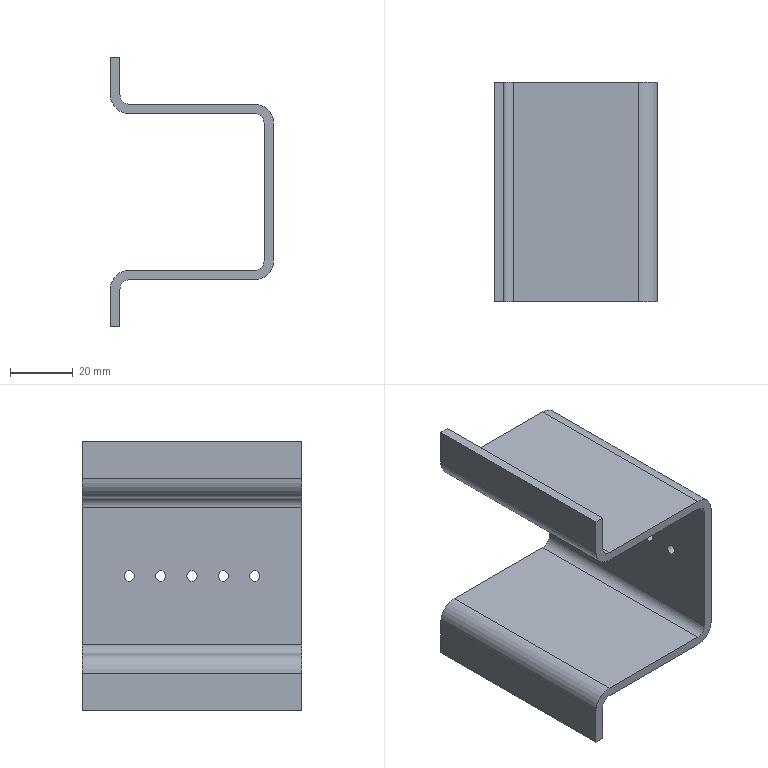Part | SolidWorks | features Fillet 2, Extrusion 1, HoleWzd 1, MoveFace 1 | 1 solid | 32 faces | box 52 x 70 x 86 mm | volume 36889 mm3 | cylinder 18 | plane 14 | commonest cylinder face diameters 3.3 x10 6 x4 12 x4
STEP:
#1=CARTESIAN_POINT('',(-1.5,55.,1.65));
#2=VERTEX_POINT('',#1);
#3=CARTESIAN_POINT('',(-1.5,55.,-1.65));
#4=VERTEX_POINT('',#3);
#5=CARTESIAN_POINT('',(-1.5,55.,0.));
#6=DIRECTION('',(1.,0.,0.));
#7=DIRECTION('',(0.,0.,-1.));
#8=AXIS2_PLACEMENT_3D('',#5,#6,#7);
#9=CIRCLE('',#8,1.65);
#10=EDGE_CURVE('',#2,#4,#9,.T.);
#11=ORIENTED_EDGE('',*,*,#10,.F.);
#12=CARTESIAN_POINT('',(1.5,55.,1.65));
#13=VERTEX_POINT('',#12);
#14=CARTESIAN_POINT('',(1.5,55.,1.65));
#15=DIRECTION('',(1.,0.,0.));
#16=VECTOR('',#15,1000.);
#17=LINE('',#14,#16);
#18=EDGE_CURVE('',#2,#13,#17,.T.);
#19=ORIENTED_EDGE('',*,*,#18,.T.);
#20=CARTESIAN_POINT('',(1.5,55.,-1.65));
#21=VERTEX_POINT('',#20);
#22=CARTESIAN_POINT('',(1.5,55.,0.));
#23=DIRECTION('',(1.,0.,0.));
#24=DIRECTION('',(0.,0.,-1.));
#25=AXIS2_PLACEMENT_3D('',#22,#23,#24);
#26=CIRCLE('',#25,1.65);
#27=EDGE_CURVE('',#13,#21,#26,.T.);
#28=ORIENTED_EDGE('',*,*,#27,.T.);
#29=CARTESIAN_POINT('',(1.5,55.,-1.65));
#30=DIRECTION('',(1.,0.,0.));
#31=VECTOR('',#30,1000.);
#32=LINE('',#29,#31);
#33=EDGE_CURVE('',#4,#21,#32,.T.);
#34=ORIENTED_EDGE('',*,*,#33,.F.);
#35=EDGE_LOOP('',(#11,#19,#28,#34));
#36=FACE_OUTER_BOUND('',#35,.T.);
#37=CARTESIAN_POINT('',(1.5,55.,0.));
#38=DIRECTION('',(1.,0.,0.));
#39=DIRECTION('',(0.,0.,-1.));
#40=AXIS2_PLACEMENT_3D('',#37,#38,#39);
#41=CYLINDRICAL_SURFACE('',#40,1.65);
#42=ADVANCED_FACE('',(#36),#41,.F.);
#43=CARTESIAN_POINT('',(-1.5,45.,1.65));
#44=VERTEX_POINT('',#43);
#45=CARTESIAN_POINT('',(-1.5,45.,-1.65));
#46=VERTEX_POINT('',#45);
#47=CARTESIAN_POINT('',(-1.5,45.,0.));
#48=DIRECTION('',(1.,0.,0.));
#49=DIRECTION('',(0.,0.,-1.));
#50=AXIS2_PLACEMENT_3D('',#47,#48,#49);
#51=CIRCLE('',#50,1.65);
#52=EDGE_CURVE('',#44,#46,#51,.T.);
#53=ORIENTED_EDGE('',*,*,#52,.F.);
#54=CARTESIAN_POINT('',(1.5,45.,1.65));
#55=VERTEX_POINT('',#54);
#56=CARTESIAN_POINT('',(1.5,45.,1.65));
#57=DIRECTION('',(1.,0.,0.));
#58=VECTOR('',#57,1000.);
#59=LINE('',#56,#58);
#60=EDGE_CURVE('',#44,#55,#59,.T.);
#61=ORIENTED_EDGE('',*,*,#60,.T.);
#62=CARTESIAN_POINT('',(1.5,45.,-1.65));
#63=VERTEX_POINT('',#62);
#64=CARTESIAN_POINT('',(1.5,45.,0.));
#65=DIRECTION('',(1.,0.,0.));
#66=DIRECTION('',(0.,0.,-1.));
#67=AXIS2_PLACEMENT_3D('',#64,#65,#66);
#68=CIRCLE('',#67,1.65);
#69=EDGE_CURVE('',#55,#63,#68,.T.);
#70=ORIENTED_EDGE('',*,*,#69,.T.);
#71=CARTESIAN_POINT('',(1.5,45.,-1.65));
#72=DIRECTION('',(1.,0.,0.));
#73=VECTOR('',#72,1000.);
#74=LINE('',#71,#73);
#75=EDGE_CURVE('',#46,#63,#74,.T.);
#76=ORIENTED_EDGE('',*,*,#75,.F.);
#77=EDGE_LOOP('',(#53,#61,#70,#76));
#78=FACE_OUTER_BOUND('',#77,.T.);
#79=CARTESIAN_POINT('',(1.5,45.,0.));
#80=DIRECTION('',(1.,0.,0.));
#81=DIRECTION('',(0.,0.,-1.));
#82=AXIS2_PLACEMENT_3D('',#79,#80,#81);
#83=CYLINDRICAL_SURFACE('',#82,1.65);
#84=ADVANCED_FACE('',(#78),#83,.F.);
#85=CARTESIAN_POINT('',(-1.5,35.,1.65));
#86=VERTEX_POINT('',#85);
#87=CARTESIAN_POINT('',(-1.5,35.,-1.65));
#88=VERTEX_POINT('',#87);
#89=CARTESIAN_POINT('',(-1.5,35.,0.));
#90=DIRECTION('',(1.,0.,0.));
#91=DIRECTION('',(0.,0.,-1.));
#92=AXIS2_PLACEMENT_3D('',#89,#90,#91);
#93=CIRCLE('',#92,1.65);
#94=EDGE_CURVE('',#86,#88,#93,.T.);
#95=ORIENTED_EDGE('',*,*,#94,.F.);
#96=CARTESIAN_POINT('',(1.5,35.,1.65));
#97=VERTEX_POINT('',#96);
#98=CARTESIAN_POINT('',(1.5,35.,1.65));
#99=DIRECTION('',(1.,0.,0.));
#100=VECTOR('',#99,1000.);
#101=LINE('',#98,#100);
#102=EDGE_CURVE('',#86,#97,#101,.T.);
#103=ORIENTED_EDGE('',*,*,#102,.T.);
#104=CARTESIAN_POINT('',(1.5,35.,-1.65));
#105=VERTEX_POINT('',#104);
#106=CARTESIAN_POINT('',(1.5,35.,0.));
#107=DIRECTION('',(1.,0.,0.));
#108=DIRECTION('',(0.,0.,-1.));
#109=AXIS2_PLACEMENT_3D('',#106,#107,#108);
#110=CIRCLE('',#109,1.65);
#111=EDGE_CURVE('',#97,#105,#110,.T.);
#112=ORIENTED_EDGE('',*,*,#111,.T.);
#113=CARTESIAN_POINT('',(1.5,35.,-1.65));
#114=DIRECTION('',(1.,0.,0.));
#115=VECTOR('',#114,1000.);
#116=LINE('',#113,#115);
#117=EDGE_CURVE('',#88,#105,#116,.T.);
#118=ORIENTED_EDGE('',*,*,#117,.F.);
#119=EDGE_LOOP('',(#95,#103,#112,#118));
#120=FACE_OUTER_BOUND('',#119,.T.);
#121=CARTESIAN_POINT('',(1.5,35.,0.));
#122=DIRECTION('',(1.,0.,0.));
#123=DIRECTION('',(0.,0.,-1.));
#124=AXIS2_PLACEMENT_3D('',#121,#122,#123);
#125=CYLINDRICAL_SURFACE('',#124,1.65);
#126=ADVANCED_FACE('',(#120),#125,.F.);
#127=CARTESIAN_POINT('',(-1.5,25.,1.65));
#128=VERTEX_POINT('',#127);
#129=CARTESIAN_POINT('',(-1.5,25.,-1.65));
#130=VERTEX_POINT('',#129);
#131=CARTESIAN_POINT('',(-1.5,25.,0.));
#132=DIRECTION('',(1.,0.,0.));
#133=DIRECTION('',(0.,0.,-1.));
#134=AXIS2_PLACEMENT_3D('',#131,#132,#133);
#135=CIRCLE('',#134,1.65);
#136=EDGE_CURVE('',#128,#130,#135,.T.);
#137=ORIENTED_EDGE('',*,*,#136,.F.);
#138=CARTESIAN_POINT('',(1.5,25.,1.65));
#139=VERTEX_POINT('',#138);
#140=CARTESIAN_POINT('',(1.5,25.,1.65));
#141=DIRECTION('',(1.,0.,0.));
#142=VECTOR('',#141,1000.);
#143=LINE('',#140,#142);
#144=EDGE_CURVE('',#128,#139,#143,.T.);
#145=ORIENTED_EDGE('',*,*,#144,.T.);
#146=CARTESIAN_POINT('',(1.5,25.,-1.65));
#147=VERTEX_POINT('',#146);
#148=CARTESIAN_POINT('',(1.5,25.,0.));
#149=DIRECTION('',(1.,0.,0.));
#150=DIRECTION('',(0.,0.,-1.));
#151=AXIS2_PLACEMENT_3D('',#148,#149,#150);
#152=CIRCLE('',#151,1.65);
#153=EDGE_CURVE('',#139,#147,#152,.T.);
#154=ORIENTED_EDGE('',*,*,#153,.T.);
#155=CARTESIAN_POINT('',(1.5,25.,-1.65));
#156=DIRECTION('',(1.,0.,0.));
#157=VECTOR('',#156,1000.);
#158=LINE('',#155,#157);
#159=EDGE_CURVE('',#130,#147,#158,.T.);
#160=ORIENTED_EDGE('',*,*,#159,.F.);
#161=EDGE_LOOP('',(#137,#145,#154,#160));
#162=FACE_OUTER_BOUND('',#161,.T.);
#163=CARTESIAN_POINT('',(1.5,25.,0.));
#164=DIRECTION('',(1.,0.,0.));
#165=DIRECTION('',(0.,0.,-1.));
#166=AXIS2_PLACEMENT_3D('',#163,#164,#165);
#167=CYLINDRICAL_SURFACE('',#166,1.65);
#168=ADVANCED_FACE('',(#162),#167,.F.);
#169=CARTESIAN_POINT('',(-1.5,15.,1.65));
#170=VERTEX_POINT('',#169);
#171=CARTESIAN_POINT('',(-1.5,15.,-1.65));
#172=VERTEX_POINT('',#171);
#173=CARTESIAN_POINT('',(-1.5,15.,0.));
#174=DIRECTION('',(1.,0.,0.));
#175=DIRECTION('',(0.,0.,-1.));
#176=AXIS2_PLACEMENT_3D('',#173,#174,#175);
#177=CIRCLE('',#176,1.65);
#178=EDGE_CURVE('',#170,#172,#177,.T.);
#179=ORIENTED_EDGE('',*,*,#178,.F.);
#180=CARTESIAN_POINT('',(1.5,15.,1.65));
#181=VERTEX_POINT('',#180);
#182=CARTESIAN_POINT('',(1.5,15.,1.65));
#183=DIRECTION('',(1.,0.,0.));
#184=VECTOR('',#183,1000.);
#185=LINE('',#182,#184);
#186=EDGE_CURVE('',#170,#181,#185,.T.);
#187=ORIENTED_EDGE('',*,*,#186,.T.);
#188=CARTESIAN_POINT('',(1.5,15.,-1.65));
#189=VERTEX_POINT('',#188);
#190=CARTESIAN_POINT('',(1.5,15.,0.));
#191=DIRECTION('',(1.,0.,0.));
#192=DIRECTION('',(0.,0.,-1.));
#193=AXIS2_PLACEMENT_3D('',#190,#191,#192);
#194=CIRCLE('',#193,1.65);
#195=EDGE_CURVE('',#181,#189,#194,.T.);
#196=ORIENTED_EDGE('',*,*,#195,.T.);
#197=CARTESIAN_POINT('',(1.5,15.,-1.65));
#198=DIRECTION('',(1.,0.,0.));
#199=VECTOR('',#198,1000.);
#200=LINE('',#197,#199);
#201=EDGE_CURVE('',#172,#189,#200,.T.);
#202=ORIENTED_EDGE('',*,*,#201,.F.);
#203=EDGE_LOOP('',(#179,#187,#196,#202));
#204=FACE_OUTER_BOUND('',#203,.T.);
#205=CARTESIAN_POINT('',(1.5,15.,0.));
#206=DIRECTION('',(1.,0.,0.));
#207=DIRECTION('',(0.,0.,-1.));
#208=AXIS2_PLACEMENT_3D('',#205,#206,#207);
#209=CYLINDRICAL_SURFACE('',#208,1.65);
#210=ADVANCED_FACE('',(#204),#209,.F.);
#211=CARTESIAN_POINT('',(-4.5,70.,-28.));
#212=VERTEX_POINT('',#211);
#213=CARTESIAN_POINT('',(-44.5,70.,-28.));
#214=VERTEX_POINT('',#213);
#215=CARTESIAN_POINT('',(1.5,70.,-28.));
#216=DIRECTION('',(-1.,0.,0.));
#217=VECTOR('',#216,1000.);
#218=LINE('',#215,#217);
#219=EDGE_CURVE('',#212,#214,#218,.T.);
#220=ORIENTED_EDGE('',*,*,#219,.F.);
#221=CARTESIAN_POINT('',(-4.5,0.,-28.));
#222=VERTEX_POINT('',#221);
#223=CARTESIAN_POINT('',(-4.5,70.,-28.));
#224=DIRECTION('',(0.,-1.,0.));
#225=VECTOR('',#224,1000.);
#226=LINE('',#223,#225);
#227=EDGE_CURVE('',#212,#222,#226,.T.);
#228=ORIENTED_EDGE('',*,*,#227,.T.);
#229=CARTESIAN_POINT('',(-44.5,0.,-28.));
#230=VERTEX_POINT('',#229);
#231=CARTESIAN_POINT('',(1.5,0.,-28.));
#232=DIRECTION('',(-1.,0.,0.));
#233=VECTOR('',#232,1000.);
#234=LINE('',#231,#233);
#235=EDGE_CURVE('',#222,#230,#234,.T.);
#236=ORIENTED_EDGE('',*,*,#235,.T.);
#237=CARTESIAN_POINT('',(-44.5,70.,-28.));
#238=DIRECTION('',(0.,1.,0.));
#239=VECTOR('',#238,1000.);
#240=LINE('',#237,#239);
#241=EDGE_CURVE('',#230,#214,#240,.T.);
#242=ORIENTED_EDGE('',*,*,#241,.T.);
#243=EDGE_LOOP('',(#220,#228,#236,#242));
#244=FACE_OUTER_BOUND('',#243,.T.);
#245=CARTESIAN_POINT('',(1.5,70.,-28.));
#246=DIRECTION('',(0.,0.,1.));
#247=DIRECTION('',(1.,0.,0.));
#248=AXIS2_PLACEMENT_3D('',#245,#246,#247);
#249=PLANE('',#248);
#250=ADVANCED_FACE('',(#244),#249,.F.);
#251=CARTESIAN_POINT('',(-47.5,70.,-31.));
#252=VERTEX_POINT('',#251);
#253=CARTESIAN_POINT('',(-47.5,70.,-43.));
#254=VERTEX_POINT('',#253);
#255=CARTESIAN_POINT('',(-47.5,70.,-28.));
#256=DIRECTION('',(0.,0.,-1.));
#257=VECTOR('',#256,1000.);
#258=LINE('',#255,#257);
#259=EDGE_CURVE('',#252,#254,#258,.T.);
#260=ORIENTED_EDGE('',*,*,#259,.F.);
#261=CARTESIAN_POINT('',(-47.5,0.,-31.));
#262=VERTEX_POINT('',#261);
#263=CARTESIAN_POINT('',(-47.5,0.,-31.));
#264=DIRECTION('',(0.,-1.,0.));
#265=VECTOR('',#264,1000.);
#266=LINE('',#263,#265);
#267=EDGE_CURVE('',#252,#262,#266,.T.);
#268=ORIENTED_EDGE('',*,*,#267,.T.);
#269=CARTESIAN_POINT('',(-47.5,0.,-43.));
#270=VERTEX_POINT('',#269);
#271=CARTESIAN_POINT('',(-47.5,0.,-28.));
#272=DIRECTION('',(0.,0.,-1.));
#273=VECTOR('',#272,1000.);
#274=LINE('',#271,#273);
#275=EDGE_CURVE('',#262,#270,#274,.T.);
#276=ORIENTED_EDGE('',*,*,#275,.T.);
#277=CARTESIAN_POINT('',(-47.5,70.,-43.));
#278=DIRECTION('',(0.,-1.,0.));
#279=VECTOR('',#278,1000.);
#280=LINE('',#277,#279);
#281=EDGE_CURVE('',#254,#270,#280,.T.);
#282=ORIENTED_EDGE('',*,*,#281,.F.);
#283=EDGE_LOOP('',(#260,#268,#276,#282));
#284=FACE_OUTER_BOUND('',#283,.T.);
#285=CARTESIAN_POINT('',(-47.5,70.,-28.));
#286=DIRECTION('',(-1.,0.,0.));
#287=DIRECTION('',(0.,0.,1.));
#288=AXIS2_PLACEMENT_3D('',#285,#286,#287);
#289=PLANE('',#288);
#290=ADVANCED_FACE('',(#284),#289,.F.);
#291=CARTESIAN_POINT('',(-50.5,0.,-43.));
#292=VERTEX_POINT('',#291);
#293=CARTESIAN_POINT('',(-35.5,0.,-43.));
#294=DIRECTION('',(-1.,0.,0.));
#295=VECTOR('',#294,1000.);
#296=LINE('',#293,#295);
#297=EDGE_CURVE('',#270,#292,#296,.T.);
#298=ORIENTED_EDGE('',*,*,#297,.T.);
#299=CARTESIAN_POINT('',(-50.5,70.,-43.));
#300=VERTEX_POINT('',#299);
#301=CARTESIAN_POINT('',(-50.5,70.,-43.));
#302=DIRECTION('',(0.,-1.,0.));
#303=VECTOR('',#302,1000.);
#304=LINE('',#301,#303);
#305=EDGE_CURVE('',#300,#292,#304,.T.);
#306=ORIENTED_EDGE('',*,*,#305,.F.);
#307=CARTESIAN_POINT('',(-35.5,70.,-43.));
#308=DIRECTION('',(-1.,0.,0.));
#309=VECTOR('',#308,1000.);
#310=LINE('',#307,#309);
#311=EDGE_CURVE('',#254,#300,#310,.T.);
#312=ORIENTED_EDGE('',*,*,#311,.F.);
#313=ORIENTED_EDGE('',*,*,#281,.T.);
#314=EDGE_LOOP('',(#298,#306,#312,#313));
#315=FACE_OUTER_BOUND('',#314,.T.);
#316=CARTESIAN_POINT('',(-35.5,70.,-43.));
#317=DIRECTION('',(0.,0.,1.));
#318=DIRECTION('',(1.,0.,0.));
#319=AXIS2_PLACEMENT_3D('',#316,#317,#318);
#320=PLANE('',#319);
#321=ADVANCED_FACE('',(#315),#320,.F.);
#322=CARTESIAN_POINT('',(-50.5,0.,-31.));
#323=VERTEX_POINT('',#322);
#324=CARTESIAN_POINT('',(-50.5,0.,-25.));
#325=DIRECTION('',(0.,0.,1.));
#326=VECTOR('',#325,1000.);
#327=LINE('',#324,#326);
#328=EDGE_CURVE('',#292,#323,#327,.T.);
#329=ORIENTED_EDGE('',*,*,#328,.T.);
#330=CARTESIAN_POINT('',(-50.5,70.,-31.));
#331=VERTEX_POINT('',#330);
#332=CARTESIAN_POINT('',(-50.5,70.,-31.));
#333=DIRECTION('',(0.,1.,0.));
#334=VECTOR('',#333,1000.);
#335=LINE('',#332,#334);
#336=EDGE_CURVE('',#323,#331,#335,.T.);
#337=ORIENTED_EDGE('',*,*,#336,.T.);
#338=CARTESIAN_POINT('',(-50.5,70.,-28.));
#339=DIRECTION('',(0.,0.,1.));
#340=VECTOR('',#339,1000.);
#341=LINE('',#338,#340);
#342=EDGE_CURVE('',#300,#331,#341,.T.);
#343=ORIENTED_EDGE('',*,*,#342,.F.);
#344=ORIENTED_EDGE('',*,*,#305,.T.);
#345=EDGE_LOOP('',(#329,#337,#343,#344));
#346=FACE_OUTER_BOUND('',#345,.T.);
#347=CARTESIAN_POINT('',(-50.5,70.,-25.));
#348=DIRECTION('',(1.,0.,0.));
#349=DIRECTION('',(0.,0.,-1.));
#350=AXIS2_PLACEMENT_3D('',#347,#348,#349);
#351=PLANE('',#350);
#352=ADVANCED_FACE('',(#346),#351,.F.);
#353=CARTESIAN_POINT('',(-44.5,70.,-25.));
#354=VERTEX_POINT('',#353);
#355=CARTESIAN_POINT('',(-4.5,70.,-25.));
#356=VERTEX_POINT('',#355);
#357=CARTESIAN_POINT('',(-1.5,70.,-25.));
#358=DIRECTION('',(1.,0.,0.));
#359=VECTOR('',#358,1000.);
#360=LINE('',#357,#359);
#361=EDGE_CURVE('',#354,#356,#360,.T.);
#362=ORIENTED_EDGE('',*,*,#361,.F.);
#363=CARTESIAN_POINT('',(-44.5,0.,-25.));
#364=VERTEX_POINT('',#363);
#365=CARTESIAN_POINT('',(-44.5,70.,-25.));
#366=DIRECTION('',(0.,-1.,0.));
#367=VECTOR('',#366,1000.);
#368=LINE('',#365,#367);
#369=EDGE_CURVE('',#354,#364,#368,.T.);
#370=ORIENTED_EDGE('',*,*,#369,.T.);
#371=CARTESIAN_POINT('',(-4.5,0.,-25.));
#372=VERTEX_POINT('',#371);
#373=CARTESIAN_POINT('',(-1.5,0.,-25.));
#374=DIRECTION('',(1.,0.,0.));
#375=VECTOR('',#374,1000.);
#376=LINE('',#373,#375);
#377=EDGE_CURVE('',#364,#372,#376,.T.);
#378=ORIENTED_EDGE('',*,*,#377,.T.);
#379=CARTESIAN_POINT('',(-4.5,70.,-25.));
#380=DIRECTION('',(0.,1.,0.));
#381=VECTOR('',#380,1000.);
#382=LINE('',#379,#381);
#383=EDGE_CURVE('',#372,#356,#382,.T.);
#384=ORIENTED_EDGE('',*,*,#383,.T.);
#385=EDGE_LOOP('',(#362,#370,#378,#384));
#386=FACE_OUTER_BOUND('',#385,.T.);
#387=CARTESIAN_POINT('',(-1.5,70.,-25.));
#388=DIRECTION('',(0.,0.,-1.));
#389=DIRECTION('',(-1.,0.,0.));
#390=AXIS2_PLACEMENT_3D('',#387,#388,#389);
#391=PLANE('',#390);
#392=ADVANCED_FACE('',(#386),#391,.F.);
#393=CARTESIAN_POINT('',(-1.5,55.,0.));
#394=DIRECTION('',(1.,0.,0.));
#395=DIRECTION('',(0.,0.,-1.));
#396=AXIS2_PLACEMENT_3D('',#393,#394,#395);
#397=CIRCLE('',#396,1.65);
#398=EDGE_CURVE('',#4,#2,#397,.T.);
#399=ORIENTED_EDGE('',*,*,#398,.T.);
#400=ORIENTED_EDGE('',*,*,#10,.T.);
#401=EDGE_LOOP('',(#399,#400));
#402=FACE_BOUND('',#401,.T.);
#403=CARTESIAN_POINT('',(-1.5,45.,0.));
#404=DIRECTION('',(1.,0.,0.));
#405=DIRECTION('',(0.,0.,-1.));
#406=AXIS2_PLACEMENT_3D('',#403,#404,#405);
#407=CIRCLE('',#406,1.65);
#408=EDGE_CURVE('',#46,#44,#407,.T.);
#409=ORIENTED_EDGE('',*,*,#408,.T.);
#410=ORIENTED_EDGE('',*,*,#52,.T.);
#411=EDGE_LOOP('',(#409,#410));
#412=FACE_BOUND('',#411,.T.);
#413=CARTESIAN_POINT('',(-1.5,35.,0.));
#414=DIRECTION('',(1.,0.,0.));
#415=DIRECTION('',(0.,0.,-1.));
#416=AXIS2_PLACEMENT_3D('',#413,#414,#415);
#417=CIRCLE('',#416,1.65);
#418=EDGE_CURVE('',#88,#86,#417,.T.);
#419=ORIENTED_EDGE('',*,*,#418,.T.);
#420=ORIENTED_EDGE('',*,*,#94,.T.);
#421=EDGE_LOOP('',(#419,#420));
#422=FACE_BOUND('',#421,.T.);
#423=CARTESIAN_POINT('',(-1.5,25.,0.));
#424=DIRECTION('',(1.,0.,0.));
#425=DIRECTION('',(0.,0.,-1.));
#426=AXIS2_PLACEMENT_3D('',#423,#424,#425);
#427=CIRCLE('',#426,1.65);
#428=EDGE_CURVE('',#130,#128,#427,.T.);
#429=ORIENTED_EDGE('',*,*,#428,.T.);
#430=ORIENTED_EDGE('',*,*,#136,.T.);
#431=EDGE_LOOP('',(#429,#430));
#432=FACE_BOUND('',#431,.T.);
#433=CARTESIAN_POINT('',(-1.5,15.,0.));
#434=DIRECTION('',(1.,0.,0.));
#435=DIRECTION('',(0.,0.,-1.));
#436=AXIS2_PLACEMENT_3D('',#433,#434,#435);
#437=CIRCLE('',#436,1.65);
#438=EDGE_CURVE('',#172,#170,#437,.T.);
#439=ORIENTED_EDGE('',*,*,#438,.T.);
#440=ORIENTED_EDGE('',*,*,#178,.T.);
#441=EDGE_LOOP('',(#439,#440));
#442=FACE_BOUND('',#441,.T.);
#443=CARTESIAN_POINT('',(-1.5,0.,-22.));
#444=VERTEX_POINT('',#443);
#445=CARTESIAN_POINT('',(-1.5,0.,22.));
#446=VERTEX_POINT('',#445);
#447=CARTESIAN_POINT('',(-1.5,0.,25.));
#448=DIRECTION('',(0.,0.,1.));
#449=VECTOR('',#448,1000.);
#450=LINE('',#447,#449);
#451=EDGE_CURVE('',#444,#446,#450,.T.);
#452=ORIENTED_EDGE('',*,*,#451,.T.);
#453=CARTESIAN_POINT('',(-1.5,70.,22.));
#454=VERTEX_POINT('',#453);
#455=CARTESIAN_POINT('',(-1.5,70.,22.));
#456=DIRECTION('',(0.,1.,0.));
#457=VECTOR('',#456,1000.);
#458=LINE('',#455,#457);
#459=EDGE_CURVE('',#446,#454,#458,.T.);
#460=ORIENTED_EDGE('',*,*,#459,.T.);
#461=CARTESIAN_POINT('',(-1.5,70.,-22.));
#462=VERTEX_POINT('',#461);
#463=CARTESIAN_POINT('',(-1.5,70.,25.));
#464=DIRECTION('',(0.,0.,1.));
#465=VECTOR('',#464,1000.);
#466=LINE('',#463,#465);
#467=EDGE_CURVE('',#462,#454,#466,.T.);
#468=ORIENTED_EDGE('',*,*,#467,.F.);
#469=CARTESIAN_POINT('',(-1.5,0.,-22.));
#470=DIRECTION('',(0.,-1.,0.));
#471=VECTOR('',#470,1000.);
#472=LINE('',#469,#471);
#473=EDGE_CURVE('',#462,#444,#472,.T.);
#474=ORIENTED_EDGE('',*,*,#473,.T.);
#475=EDGE_LOOP('',(#452,#460,#468,#474));
#476=FACE_OUTER_BOUND('',#475,.T.);
#477=CARTESIAN_POINT('',(-1.5,70.,25.));
#478=DIRECTION('',(1.,0.,0.));
#479=DIRECTION('',(0.,0.,-1.));
#480=AXIS2_PLACEMENT_3D('',#477,#478,#479);
#481=PLANE('',#480);
#482=ADVANCED_FACE('',(#402,#412,#422,#432,#442,#476),#481,.F.);
#483=CARTESIAN_POINT('',(-4.5,0.,25.));
#484=VERTEX_POINT('',#483);
#485=CARTESIAN_POINT('',(-44.5,0.,25.));
#486=VERTEX_POINT('',#485);
#487=CARTESIAN_POINT('',(-1.5,0.,25.));
#488=DIRECTION('',(-1.,0.,0.));
#489=VECTOR('',#488,1000.);
#490=LINE('',#487,#489);
#491=EDGE_CURVE('',#484,#486,#490,.T.);
#492=ORIENTED_EDGE('',*,*,#491,.T.);
#493=CARTESIAN_POINT('',(-44.5,70.,25.));
#494=VERTEX_POINT('',#493);
#495=CARTESIAN_POINT('',(-44.5,70.,25.));
#496=DIRECTION('',(0.,1.,0.));
#497=VECTOR('',#496,1000.);
#498=LINE('',#495,#497);
#499=EDGE_CURVE('',#486,#494,#498,.T.);
#500=ORIENTED_EDGE('',*,*,#499,.T.);
#501=CARTESIAN_POINT('',(-4.5,70.,25.));
#502=VERTEX_POINT('',#501);
#503=CARTESIAN_POINT('',(-1.5,70.,25.));
#504=DIRECTION('',(-1.,0.,0.));
#505=VECTOR('',#504,1000.);
#506=LINE('',#503,#505);
#507=EDGE_CURVE('',#502,#494,#506,.T.);
#508=ORIENTED_EDGE('',*,*,#507,.F.);
#509=CARTESIAN_POINT('',(-4.5,0.,25.));
#510=DIRECTION('',(0.,-1.,0.));
#511=VECTOR('',#510,1000.);
#512=LINE('',#509,#511);
#513=EDGE_CURVE('',#502,#484,#512,.T.);
#514=ORIENTED_EDGE('',*,*,#513,.T.);
#515=EDGE_LOOP('',(#492,#500,#508,#514));
#516=FACE_OUTER_BOUND('',#515,.T.);
#517=CARTESIAN_POINT('',(-1.5,70.,25.));
#518=DIRECTION('',(0.,0.,1.));
#519=DIRECTION('',(1.,0.,0.));
#520=AXIS2_PLACEMENT_3D('',#517,#518,#519);
#521=PLANE('',#520);
#522=ADVANCED_FACE('',(#516),#521,.F.);
#523=CARTESIAN_POINT('',(-50.5,70.,31.));
#524=VERTEX_POINT('',#523);
#525=CARTESIAN_POINT('',(-50.5,70.,43.));
#526=VERTEX_POINT('',#525);
#527=CARTESIAN_POINT('',(-50.5,70.,25.));
#528=DIRECTION('',(0.,0.,1.));
#529=VECTOR('',#528,1000.);
#530=LINE('',#527,#529);
#531=EDGE_CURVE('',#524,#526,#530,.T.);
#532=ORIENTED_EDGE('',*,*,#531,.F.);
#533=CARTESIAN_POINT('',(-50.5,0.,31.));
#534=VERTEX_POINT('',#533);
#535=CARTESIAN_POINT('',(-50.5,70.,31.));
#536=DIRECTION('',(0.,-1.,0.));
#537=VECTOR('',#536,1000.);
#538=LINE('',#535,#537);
#539=EDGE_CURVE('',#524,#534,#538,.T.);
#540=ORIENTED_EDGE('',*,*,#539,.T.);
#541=CARTESIAN_POINT('',(-50.5,0.,43.));
#542=VERTEX_POINT('',#541);
#543=CARTESIAN_POINT('',(-50.5,0.,28.));
#544=DIRECTION('',(0.,0.,1.));
#545=VECTOR('',#544,1000.);
#546=LINE('',#543,#545);
#547=EDGE_CURVE('',#534,#542,#546,.T.);
#548=ORIENTED_EDGE('',*,*,#547,.T.);
#549=CARTESIAN_POINT('',(-50.5,70.,43.));
#550=DIRECTION('',(0.,-1.,0.));
#551=VECTOR('',#550,1000.);
#552=LINE('',#549,#551);
#553=EDGE_CURVE('',#526,#542,#552,.T.);
#554=ORIENTED_EDGE('',*,*,#553,.F.);
#555=EDGE_LOOP('',(#532,#540,#548,#554));
#556=FACE_OUTER_BOUND('',#555,.T.);
#557=CARTESIAN_POINT('',(-50.5,70.,28.));
#558=DIRECTION('',(1.,0.,0.));
#559=DIRECTION('',(0.,0.,-1.));
#560=AXIS2_PLACEMENT_3D('',#557,#558,#559);
#561=PLANE('',#560);
#562=ADVANCED_FACE('',(#556),#561,.F.);
#563=CARTESIAN_POINT('',(-47.5,0.,43.));
#564=VERTEX_POINT('',#563);
#565=CARTESIAN_POINT('',(-35.5,0.,43.));
#566=DIRECTION('',(1.,0.,0.));
#567=VECTOR('',#566,1000.);
#568=LINE('',#565,#567);
#569=EDGE_CURVE('',#542,#564,#568,.T.);
#570=ORIENTED_EDGE('',*,*,#569,.T.);
#571=CARTESIAN_POINT('',(-47.5,70.,43.));
#572=VERTEX_POINT('',#571);
#573=CARTESIAN_POINT('',(-47.5,70.,43.));
#574=DIRECTION('',(0.,-1.,0.));
#575=VECTOR('',#574,1000.);
#576=LINE('',#573,#575);
#577=EDGE_CURVE('',#572,#564,#576,.T.);
#578=ORIENTED_EDGE('',*,*,#577,.F.);
#579=CARTESIAN_POINT('',(-35.5,70.,43.));
#580=DIRECTION('',(1.,0.,0.));
#581=VECTOR('',#580,1000.);
#582=LINE('',#579,#581);
#583=EDGE_CURVE('',#526,#572,#582,.T.);
#584=ORIENTED_EDGE('',*,*,#583,.F.);
#585=ORIENTED_EDGE('',*,*,#553,.T.);
#586=EDGE_LOOP('',(#570,#578,#584,#585));
#587=FACE_OUTER_BOUND('',#586,.T.);
#588=CARTESIAN_POINT('',(-35.5,70.,43.));
#589=DIRECTION('',(0.,0.,-1.));
#590=DIRECTION('',(-1.,0.,0.));
#591=AXIS2_PLACEMENT_3D('',#588,#589,#590);
#592=PLANE('',#591);
#593=ADVANCED_FACE('',(#587),#592,.F.);
#594=CARTESIAN_POINT('',(-47.5,0.,31.));
#595=VERTEX_POINT('',#594);
#596=CARTESIAN_POINT('',(-47.5,0.,28.));
#597=DIRECTION('',(0.,0.,-1.));
#598=VECTOR('',#597,1000.);
#599=LINE('',#596,#598);
#600=EDGE_CURVE('',#564,#595,#599,.T.);
#601=ORIENTED_EDGE('',*,*,#600,.T.);
#602=CARTESIAN_POINT('',(-47.5,70.,31.));
#603=VERTEX_POINT('',#602);
#604=CARTESIAN_POINT('',(-47.5,70.,31.));
#605=DIRECTION('',(0.,1.,0.));
#606=VECTOR('',#605,1000.);
#607=LINE('',#604,#606);
#608=EDGE_CURVE('',#595,#603,#607,.T.);
#609=ORIENTED_EDGE('',*,*,#608,.T.);
#610=CARTESIAN_POINT('',(-47.5,70.,28.));
#611=DIRECTION('',(0.,0.,-1.));
#612=VECTOR('',#611,1000.);
#613=LINE('',#610,#612);
#614=EDGE_CURVE('',#572,#603,#613,.T.);
#615=ORIENTED_EDGE('',*,*,#614,.F.);
#616=ORIENTED_EDGE('',*,*,#577,.T.);
#617=EDGE_LOOP('',(#601,#609,#615,#616));
#618=FACE_OUTER_BOUND('',#617,.T.);
#619=CARTESIAN_POINT('',(-47.5,70.,28.));
#620=DIRECTION('',(-1.,0.,0.));
#621=DIRECTION('',(0.,0.,1.));
#622=AXIS2_PLACEMENT_3D('',#619,#620,#621);
#623=PLANE('',#622);
#624=ADVANCED_FACE('',(#618),#623,.F.);
#625=CARTESIAN_POINT('',(-44.5,0.,28.));
#626=VERTEX_POINT('',#625);
#627=CARTESIAN_POINT('',(-4.5,0.,28.));
#628=VERTEX_POINT('',#627);
#629=CARTESIAN_POINT('',(1.5,0.,28.));
#630=DIRECTION('',(1.,0.,0.));
#631=VECTOR('',#630,1000.);
#632=LINE('',#629,#631);
#633=EDGE_CURVE('',#626,#628,#632,.T.);
#634=ORIENTED_EDGE('',*,*,#633,.T.);
#635=CARTESIAN_POINT('',(-4.5,70.,28.));
#636=VERTEX_POINT('',#635);
#637=CARTESIAN_POINT('',(-4.5,70.,28.));
#638=DIRECTION('',(0.,1.,0.));
#639=VECTOR('',#638,1000.);
#640=LINE('',#637,#639);
#641=EDGE_CURVE('',#628,#636,#640,.T.);
#642=ORIENTED_EDGE('',*,*,#641,.T.);
#643=CARTESIAN_POINT('',(-44.5,70.,28.));
#644=VERTEX_POINT('',#643);
#645=CARTESIAN_POINT('',(1.5,70.,28.));
#646=DIRECTION('',(1.,0.,0.));
#647=VECTOR('',#646,1000.);
#648=LINE('',#645,#647);
#649=EDGE_CURVE('',#644,#636,#648,.T.);
#650=ORIENTED_EDGE('',*,*,#649,.F.);
#651=CARTESIAN_POINT('',(-44.5,0.,28.));
#652=DIRECTION('',(0.,-1.,0.));
#653=VECTOR('',#652,1000.);
#654=LINE('',#651,#653);
#655=EDGE_CURVE('',#644,#626,#654,.T.);
#656=ORIENTED_EDGE('',*,*,#655,.T.);
#657=EDGE_LOOP('',(#634,#642,#650,#656));
#658=FACE_OUTER_BOUND('',#657,.T.);
#659=CARTESIAN_POINT('',(1.5,70.,28.));
#660=DIRECTION('',(0.,0.,-1.));
#661=DIRECTION('',(-1.,0.,0.));
#662=AXIS2_PLACEMENT_3D('',#659,#660,#661);
#663=PLANE('',#662);
#664=ADVANCED_FACE('',(#658),#663,.F.);
#665=CARTESIAN_POINT('',(1.5,55.,0.));
#666=DIRECTION('',(1.,0.,0.));
#667=DIRECTION('',(0.,0.,-1.));
#668=AXIS2_PLACEMENT_3D('',#665,#666,#667);
#669=CIRCLE('',#668,1.65);
#670=EDGE_CURVE('',#21,#13,#669,.T.);
#671=ORIENTED_EDGE('',*,*,#670,.F.);
#672=ORIENTED_EDGE('',*,*,#27,.F.);
#673=EDGE_LOOP('',(#671,#672));
#674=FACE_BOUND('',#673,.T.);
#675=CARTESIAN_POINT('',(1.5,45.,0.));
#676=DIRECTION('',(1.,0.,0.));
#677=DIRECTION('',(0.,0.,-1.));
#678=AXIS2_PLACEMENT_3D('',#675,#676,#677);
#679=CIRCLE('',#678,1.65);
#680=EDGE_CURVE('',#63,#55,#679,.T.);
#681=ORIENTED_EDGE('',*,*,#680,.F.);
#682=ORIENTED_EDGE('',*,*,#69,.F.);
#683=EDGE_LOOP('',(#681,#682));
#684=FACE_BOUND('',#683,.T.);
#685=CARTESIAN_POINT('',(1.5,35.,0.));
#686=DIRECTION('',(1.,0.,0.));
#687=DIRECTION('',(0.,0.,-1.));
#688=AXIS2_PLACEMENT_3D('',#685,#686,#687);
#689=CIRCLE('',#688,1.65);
#690=EDGE_CURVE('',#105,#97,#689,.T.);
#691=ORIENTED_EDGE('',*,*,#690,.F.);
#692=ORIENTED_EDGE('',*,*,#111,.F.);
#693=EDGE_LOOP('',(#691,#692));
#694=FACE_BOUND('',#693,.T.);
#695=CARTESIAN_POINT('',(1.5,25.,0.));
#696=DIRECTION('',(1.,0.,0.));
#697=DIRECTION('',(0.,0.,-1.));
#698=AXIS2_PLACEMENT_3D('',#695,#696,#697);
#699=CIRCLE('',#698,1.65);
#700=EDGE_CURVE('',#147,#139,#699,.T.);
#701=ORIENTED_EDGE('',*,*,#700,.F.);
#702=ORIENTED_EDGE('',*,*,#153,.F.);
#703=EDGE_LOOP('',(#701,#702));
#704=FACE_BOUND('',#703,.T.);
#705=CARTESIAN_POINT('',(1.5,15.,0.));
#706=DIRECTION('',(1.,0.,0.));
#707=DIRECTION('',(0.,0.,-1.));
#708=AXIS2_PLACEMENT_3D('',#705,#706,#707);
#709=CIRCLE('',#708,1.65);
#710=EDGE_CURVE('',#189,#181,#709,.T.);
#711=ORIENTED_EDGE('',*,*,#710,.F.);
#712=ORIENTED_EDGE('',*,*,#195,.F.);
#713=EDGE_LOOP('',(#711,#712));
#714=FACE_BOUND('',#713,.T.);
#715=CARTESIAN_POINT('',(1.5,70.,22.));
#716=VERTEX_POINT('',#715);
#717=CARTESIAN_POINT('',(1.5,70.,-22.));
#718=VERTEX_POINT('',#717);
#719=CARTESIAN_POINT('',(1.5,70.,-25.));
#720=DIRECTION('',(0.,0.,-1.));
#721=VECTOR('',#720,1000.);
#722=LINE('',#719,#721);
#723=EDGE_CURVE('',#716,#718,#722,.T.);
#724=ORIENTED_EDGE('',*,*,#723,.F.);
#725=CARTESIAN_POINT('',(1.5,0.,22.));
#726=VERTEX_POINT('',#725);
#727=CARTESIAN_POINT('',(1.5,70.,22.));
#728=DIRECTION('',(0.,-1.,0.));
#729=VECTOR('',#728,1000.);
#730=LINE('',#727,#729);
#731=EDGE_CURVE('',#716,#726,#730,.T.);
#732=ORIENTED_EDGE('',*,*,#731,.T.);
#733=CARTESIAN_POINT('',(1.5,0.,-22.));
#734=VERTEX_POINT('',#733);
#735=CARTESIAN_POINT('',(1.5,0.,25.));
#736=DIRECTION('',(0.,0.,-1.));
#737=VECTOR('',#736,1000.);
#738=LINE('',#735,#737);
#739=EDGE_CURVE('',#726,#734,#738,.T.);
#740=ORIENTED_EDGE('',*,*,#739,.T.);
#741=CARTESIAN_POINT('',(1.5,70.,-22.));
#742=DIRECTION('',(0.,1.,0.));
#743=VECTOR('',#742,1000.);
#744=LINE('',#741,#743);
#745=EDGE_CURVE('',#734,#718,#744,.T.);
#746=ORIENTED_EDGE('',*,*,#745,.T.);
#747=EDGE_LOOP('',(#724,#732,#740,#746));
#748=FACE_OUTER_BOUND('',#747,.T.);
#749=CARTESIAN_POINT('',(1.5,70.,25.));
#750=DIRECTION('',(-1.,0.,0.));
#751=DIRECTION('',(0.,0.,1.));
#752=AXIS2_PLACEMENT_3D('',#749,#750,#751);
#753=PLANE('',#752);
#754=ADVANCED_FACE('',(#674,#684,#694,#704,#714,#748),#753,.F.);
#755=ORIENTED_EDGE('',*,*,#507,.T.);
#756=CARTESIAN_POINT('',(-44.5,70.,31.));
#757=DIRECTION('',(0.,1.,0.));
#758=DIRECTION('',(0.,0.,1.));
#759=AXIS2_PLACEMENT_3D('',#756,#757,#758);
#760=CIRCLE('',#759,6.);
#761=EDGE_CURVE('',#494,#524,#760,.T.);
#762=ORIENTED_EDGE('',*,*,#761,.T.);
#763=ORIENTED_EDGE('',*,*,#531,.T.);
#764=ORIENTED_EDGE('',*,*,#583,.T.);
#765=ORIENTED_EDGE('',*,*,#614,.T.);
#766=CARTESIAN_POINT('',(-44.5,70.,31.));
#767=DIRECTION('',(0.,-1.,0.));
#768=DIRECTION('',(0.,0.,1.));
#769=AXIS2_PLACEMENT_3D('',#766,#767,#768);
#770=CIRCLE('',#769,3.);
#771=EDGE_CURVE('',#603,#644,#770,.T.);
#772=ORIENTED_EDGE('',*,*,#771,.T.);
#773=ORIENTED_EDGE('',*,*,#649,.T.);
#774=CARTESIAN_POINT('',(-4.5,70.,22.));
#775=DIRECTION('',(0.,1.,0.));
#776=DIRECTION('',(0.,0.,1.));
#777=AXIS2_PLACEMENT_3D('',#774,#775,#776);
#778=CIRCLE('',#777,6.);
#779=EDGE_CURVE('',#636,#716,#778,.T.);
#780=ORIENTED_EDGE('',*,*,#779,.T.);
#781=ORIENTED_EDGE('',*,*,#723,.T.);
#782=CARTESIAN_POINT('',(-4.5,70.,-22.));
#783=DIRECTION('',(0.,1.,0.));
#784=DIRECTION('',(0.,0.,1.));
#785=AXIS2_PLACEMENT_3D('',#782,#783,#784);
#786=CIRCLE('',#785,6.);
#787=EDGE_CURVE('',#718,#212,#786,.T.);
#788=ORIENTED_EDGE('',*,*,#787,.T.);
#789=ORIENTED_EDGE('',*,*,#219,.T.);
#790=CARTESIAN_POINT('',(-44.5,70.,-31.));
#791=DIRECTION('',(0.,-1.,0.));
#792=DIRECTION('',(0.,0.,1.));
#793=AXIS2_PLACEMENT_3D('',#790,#791,#792);
#794=CIRCLE('',#793,3.);
#795=EDGE_CURVE('',#214,#252,#794,.T.);
#796=ORIENTED_EDGE('',*,*,#795,.T.);
#797=ORIENTED_EDGE('',*,*,#259,.T.);
#798=ORIENTED_EDGE('',*,*,#311,.T.);
#799=ORIENTED_EDGE('',*,*,#342,.T.);
#800=CARTESIAN_POINT('',(-44.5,70.,-31.));
#801=DIRECTION('',(0.,1.,0.));
#802=DIRECTION('',(0.,0.,1.));
#803=AXIS2_PLACEMENT_3D('',#800,#801,#802);
#804=CIRCLE('',#803,6.);
#805=EDGE_CURVE('',#331,#354,#804,.T.);
#806=ORIENTED_EDGE('',*,*,#805,.T.);
#807=ORIENTED_EDGE('',*,*,#361,.T.);
#808=CARTESIAN_POINT('',(-4.5,70.,-22.));
#809=DIRECTION('',(0.,-1.,0.));
#810=DIRECTION('',(0.,0.,1.));
#811=AXIS2_PLACEMENT_3D('',#808,#809,#810);
#812=CIRCLE('',#811,3.);
#813=EDGE_CURVE('',#356,#462,#812,.T.);
#814=ORIENTED_EDGE('',*,*,#813,.T.);
#815=ORIENTED_EDGE('',*,*,#467,.T.);
#816=CARTESIAN_POINT('',(-4.5,70.,22.));
#817=DIRECTION('',(0.,-1.,0.));
#818=DIRECTION('',(0.,0.,1.));
#819=AXIS2_PLACEMENT_3D('',#816,#817,#818);
#820=CIRCLE('',#819,3.);
#821=EDGE_CURVE('',#454,#502,#820,.T.);
#822=ORIENTED_EDGE('',*,*,#821,.T.);
#823=EDGE_LOOP('',(#755,#762,#763,#764,#765,#772,#773,#780,#781,#788,#789,#796,#797,#798,#799,#806,#807,#814,#815,#822));
#824=FACE_OUTER_BOUND('',#823,.T.);
#825=CARTESIAN_POINT('',(0.,70.,0.));
#826=DIRECTION('',(0.,1.,0.));
#827=DIRECTION('',(0.,0.,1.));
#828=AXIS2_PLACEMENT_3D('',#825,#826,#827);
#829=PLANE('',#828);
#830=ADVANCED_FACE('',(#824),#829,.T.);
#831=ORIENTED_EDGE('',*,*,#547,.F.);
#832=CARTESIAN_POINT('',(-44.5,0.,31.));
#833=DIRECTION('',(0.,-1.,0.));
#834=DIRECTION('',(0.,0.,1.));
#835=AXIS2_PLACEMENT_3D('',#832,#833,#834);
#836=CIRCLE('',#835,6.);
#837=EDGE_CURVE('',#534,#486,#836,.T.);
#838=ORIENTED_EDGE('',*,*,#837,.T.);
#839=ORIENTED_EDGE('',*,*,#491,.F.);
#840=CARTESIAN_POINT('',(-4.5,0.,22.));
#841=DIRECTION('',(0.,1.,0.));
#842=DIRECTION('',(0.,0.,1.));
#843=AXIS2_PLACEMENT_3D('',#840,#841,#842);
#844=CIRCLE('',#843,3.);
#845=EDGE_CURVE('',#484,#446,#844,.T.);
#846=ORIENTED_EDGE('',*,*,#845,.T.);
#847=ORIENTED_EDGE('',*,*,#451,.F.);
#848=CARTESIAN_POINT('',(-4.5,0.,-22.));
#849=DIRECTION('',(0.,1.,0.));
#850=DIRECTION('',(0.,0.,1.));
#851=AXIS2_PLACEMENT_3D('',#848,#849,#850);
#852=CIRCLE('',#851,3.);
#853=EDGE_CURVE('',#444,#372,#852,.T.);
#854=ORIENTED_EDGE('',*,*,#853,.T.);
#855=ORIENTED_EDGE('',*,*,#377,.F.);
#856=CARTESIAN_POINT('',(-44.5,0.,-31.));
#857=DIRECTION('',(0.,-1.,0.));
#858=DIRECTION('',(0.,0.,1.));
#859=AXIS2_PLACEMENT_3D('',#856,#857,#858);
#860=CIRCLE('',#859,6.);
#861=EDGE_CURVE('',#364,#323,#860,.T.);
#862=ORIENTED_EDGE('',*,*,#861,.T.);
#863=ORIENTED_EDGE('',*,*,#328,.F.);
#864=ORIENTED_EDGE('',*,*,#297,.F.);
#865=ORIENTED_EDGE('',*,*,#275,.F.);
#866=CARTESIAN_POINT('',(-44.5,0.,-31.));
#867=DIRECTION('',(0.,1.,0.));
#868=DIRECTION('',(0.,0.,1.));
#869=AXIS2_PLACEMENT_3D('',#866,#867,#868);
#870=CIRCLE('',#869,3.);
#871=EDGE_CURVE('',#262,#230,#870,.T.);
#872=ORIENTED_EDGE('',*,*,#871,.T.);
#873=ORIENTED_EDGE('',*,*,#235,.F.);
#874=CARTESIAN_POINT('',(-4.5,0.,-22.));
#875=DIRECTION('',(0.,-1.,0.));
#876=DIRECTION('',(0.,0.,1.));
#877=AXIS2_PLACEMENT_3D('',#874,#875,#876);
#878=CIRCLE('',#877,6.);
#879=EDGE_CURVE('',#222,#734,#878,.T.);
#880=ORIENTED_EDGE('',*,*,#879,.T.);
#881=ORIENTED_EDGE('',*,*,#739,.F.);
#882=CARTESIAN_POINT('',(-4.5,0.,22.));
#883=DIRECTION('',(0.,-1.,0.));
#884=DIRECTION('',(0.,0.,1.));
#885=AXIS2_PLACEMENT_3D('',#882,#883,#884);
#886=CIRCLE('',#885,6.);
#887=EDGE_CURVE('',#726,#628,#886,.T.);
#888=ORIENTED_EDGE('',*,*,#887,.T.);
#889=ORIENTED_EDGE('',*,*,#633,.F.);
#890=CARTESIAN_POINT('',(-44.5,0.,31.));
#891=DIRECTION('',(0.,1.,0.));
#892=DIRECTION('',(0.,0.,1.));
#893=AXIS2_PLACEMENT_3D('',#890,#891,#892);
#894=CIRCLE('',#893,3.);
#895=EDGE_CURVE('',#626,#595,#894,.T.);
#896=ORIENTED_EDGE('',*,*,#895,.T.);
#897=ORIENTED_EDGE('',*,*,#600,.F.);
#898=ORIENTED_EDGE('',*,*,#569,.F.);
#899=EDGE_LOOP('',(#831,#838,#839,#846,#847,#854,#855,#862,#863,#864,#865,#872,#873,#880,#881,#888,#889,#896,#897,#898));
#900=FACE_OUTER_BOUND('',#899,.T.);
#901=CARTESIAN_POINT('',(0.,0.,0.));
#902=DIRECTION('',(0.,1.,0.));
#903=DIRECTION('',(0.,0.,1.));
#904=AXIS2_PLACEMENT_3D('',#901,#902,#903);
#905=PLANE('',#904);
#906=ADVANCED_FACE('',(#900),#905,.F.);
#907=ORIENTED_EDGE('',*,*,#771,.F.);
#908=ORIENTED_EDGE('',*,*,#608,.F.);
#909=ORIENTED_EDGE('',*,*,#895,.F.);
#910=ORIENTED_EDGE('',*,*,#655,.F.);
#911=EDGE_LOOP('',(#907,#908,#909,#910));
#912=FACE_OUTER_BOUND('',#911,.T.);
#913=CARTESIAN_POINT('',(-44.5,70.,31.));
#914=DIRECTION('',(0.,1.,0.));
#915=DIRECTION('',(0.,0.,1.));
#916=AXIS2_PLACEMENT_3D('',#913,#914,#915);
#917=CYLINDRICAL_SURFACE('',#916,3.);
#918=ADVANCED_FACE('',(#912),#917,.F.);
#919=ORIENTED_EDGE('',*,*,#821,.F.);
#920=ORIENTED_EDGE('',*,*,#459,.F.);
#921=ORIENTED_EDGE('',*,*,#845,.F.);
#922=ORIENTED_EDGE('',*,*,#513,.F.);
#923=EDGE_LOOP('',(#919,#920,#921,#922));
#924=FACE_OUTER_BOUND('',#923,.T.);
#925=CARTESIAN_POINT('',(-4.5,70.,22.));
#926=DIRECTION('',(0.,1.,0.));
#927=DIRECTION('',(0.,0.,1.));
#928=AXIS2_PLACEMENT_3D('',#925,#926,#927);
#929=CYLINDRICAL_SURFACE('',#928,3.);
#930=ADVANCED_FACE('',(#924),#929,.F.);
#931=ORIENTED_EDGE('',*,*,#813,.F.);
#932=ORIENTED_EDGE('',*,*,#383,.F.);
#933=ORIENTED_EDGE('',*,*,#853,.F.);
#934=ORIENTED_EDGE('',*,*,#473,.F.);
#935=EDGE_LOOP('',(#931,#932,#933,#934));
#936=FACE_OUTER_BOUND('',#935,.T.);
#937=CARTESIAN_POINT('',(-4.5,70.,-22.));
#938=DIRECTION('',(0.,1.,0.));
#939=DIRECTION('',(0.,0.,1.));
#940=AXIS2_PLACEMENT_3D('',#937,#938,#939);
#941=CYLINDRICAL_SURFACE('',#940,3.);
#942=ADVANCED_FACE('',(#936),#941,.F.);
#943=ORIENTED_EDGE('',*,*,#795,.F.);
#944=ORIENTED_EDGE('',*,*,#241,.F.);
#945=ORIENTED_EDGE('',*,*,#871,.F.);
#946=ORIENTED_EDGE('',*,*,#267,.F.);
#947=EDGE_LOOP('',(#943,#944,#945,#946));
#948=FACE_OUTER_BOUND('',#947,.T.);
#949=CARTESIAN_POINT('',(-44.5,70.,-31.));
#950=DIRECTION('',(0.,1.,0.));
#951=DIRECTION('',(0.,0.,1.));
#952=AXIS2_PLACEMENT_3D('',#949,#950,#951);
#953=CYLINDRICAL_SURFACE('',#952,3.);
#954=ADVANCED_FACE('',(#948),#953,.F.);
#955=ORIENTED_EDGE('',*,*,#761,.F.);
#956=ORIENTED_EDGE('',*,*,#499,.F.);
#957=ORIENTED_EDGE('',*,*,#837,.F.);
#958=ORIENTED_EDGE('',*,*,#539,.F.);
#959=EDGE_LOOP('',(#955,#956,#957,#958));
#960=FACE_OUTER_BOUND('',#959,.T.);
#961=CARTESIAN_POINT('',(-44.5,70.,31.));
#962=DIRECTION('',(0.,-1.,0.));
#963=DIRECTION('',(0.,0.,-1.));
#964=AXIS2_PLACEMENT_3D('',#961,#962,#963);
#965=CYLINDRICAL_SURFACE('',#964,6.);
#966=ADVANCED_FACE('',(#960),#965,.T.);
#967=ORIENTED_EDGE('',*,*,#779,.F.);
#968=ORIENTED_EDGE('',*,*,#641,.F.);
#969=ORIENTED_EDGE('',*,*,#887,.F.);
#970=ORIENTED_EDGE('',*,*,#731,.F.);
#971=EDGE_LOOP('',(#967,#968,#969,#970));
#972=FACE_OUTER_BOUND('',#971,.T.);
#973=CARTESIAN_POINT('',(-4.5,70.,22.));
#974=DIRECTION('',(0.,-1.,0.));
#975=DIRECTION('',(0.,0.,-1.));
#976=AXIS2_PLACEMENT_3D('',#973,#974,#975);
#977=CYLINDRICAL_SURFACE('',#976,6.);
#978=ADVANCED_FACE('',(#972),#977,.T.);
#979=ORIENTED_EDGE('',*,*,#787,.F.);
#980=ORIENTED_EDGE('',*,*,#745,.F.);
#981=ORIENTED_EDGE('',*,*,#879,.F.);
#982=ORIENTED_EDGE('',*,*,#227,.F.);
#983=EDGE_LOOP('',(#979,#980,#981,#982));
#984=FACE_OUTER_BOUND('',#983,.T.);
#985=CARTESIAN_POINT('',(-4.5,70.,-22.));
#986=DIRECTION('',(0.,-1.,0.));
#987=DIRECTION('',(0.,0.,-1.));
#988=AXIS2_PLACEMENT_3D('',#985,#986,#987);
#989=CYLINDRICAL_SURFACE('',#988,6.);
#990=ADVANCED_FACE('',(#984),#989,.T.);
#991=ORIENTED_EDGE('',*,*,#805,.F.);
#992=ORIENTED_EDGE('',*,*,#336,.F.);
#993=ORIENTED_EDGE('',*,*,#861,.F.);
#994=ORIENTED_EDGE('',*,*,#369,.F.);
#995=EDGE_LOOP('',(#991,#992,#993,#994));
#996=FACE_OUTER_BOUND('',#995,.T.);
#997=CARTESIAN_POINT('',(-44.5,70.,-31.));
#998=DIRECTION('',(0.,-1.,0.));
#999=DIRECTION('',(0.,0.,-1.));
#1000=AXIS2_PLACEMENT_3D('',#997,#998,#999);
#1001=CYLINDRICAL_SURFACE('',#1000,6.);
#1002=ADVANCED_FACE('',(#996),#1001,.T.);
#1003=ORIENTED_EDGE('',*,*,#186,.F.);
#1004=ORIENTED_EDGE('',*,*,#438,.F.);
#1005=ORIENTED_EDGE('',*,*,#201,.T.);
#1006=ORIENTED_EDGE('',*,*,#710,.T.);
#1007=EDGE_LOOP('',(#1003,#1004,#1005,#1006));
#1008=FACE_OUTER_BOUND('',#1007,.T.);
#1009=CARTESIAN_POINT('',(1.5,15.,0.));
#1010=DIRECTION('',(1.,0.,0.));
#1011=DIRECTION('',(0.,0.,-1.));
#1012=AXIS2_PLACEMENT_3D('',#1009,#1010,#1011);
#1013=CYLINDRICAL_SURFACE('',#1012,1.65);
#1014=ADVANCED_FACE('',(#1008),#1013,.F.);
#1015=ORIENTED_EDGE('',*,*,#144,.F.);
#1016=ORIENTED_EDGE('',*,*,#428,.F.);
#1017=ORIENTED_EDGE('',*,*,#159,.T.);
#1018=ORIENTED_EDGE('',*,*,#700,.T.);
#1019=EDGE_LOOP('',(#1015,#1016,#1017,#1018));
#1020=FACE_OUTER_BOUND('',#1019,.T.);
#1021=CARTESIAN_POINT('',(1.5,25.,0.));
#1022=DIRECTION('',(1.,0.,0.));
#1023=DIRECTION('',(0.,0.,-1.));
#1024=AXIS2_PLACEMENT_3D('',#1021,#1022,#1023);
#1025=CYLINDRICAL_SURFACE('',#1024,1.65);
#1026=ADVANCED_FACE('',(#1020),#1025,.F.);
#1027=ORIENTED_EDGE('',*,*,#102,.F.);
#1028=ORIENTED_EDGE('',*,*,#418,.F.);
#1029=ORIENTED_EDGE('',*,*,#117,.T.);
#1030=ORIENTED_EDGE('',*,*,#690,.T.);
#1031=EDGE_LOOP('',(#1027,#1028,#1029,#1030));
#1032=FACE_OUTER_BOUND('',#1031,.T.);
#1033=CARTESIAN_POINT('',(1.5,35.,0.));
#1034=DIRECTION('',(1.,0.,0.));
#1035=DIRECTION('',(0.,0.,-1.));
#1036=AXIS2_PLACEMENT_3D('',#1033,#1034,#1035);
#1037=CYLINDRICAL_SURFACE('',#1036,1.65);
#1038=ADVANCED_FACE('',(#1032),#1037,.F.);
#1039=ORIENTED_EDGE('',*,*,#60,.F.);
#1040=ORIENTED_EDGE('',*,*,#408,.F.);
#1041=ORIENTED_EDGE('',*,*,#75,.T.);
#1042=ORIENTED_EDGE('',*,*,#680,.T.);
#1043=EDGE_LOOP('',(#1039,#1040,#1041,#1042));
#1044=FACE_OUTER_BOUND('',#1043,.T.);
#1045=CARTESIAN_POINT('',(1.5,45.,0.));
#1046=DIRECTION('',(1.,0.,0.));
#1047=DIRECTION('',(0.,0.,-1.));
#1048=AXIS2_PLACEMENT_3D('',#1045,#1046,#1047);
#1049=CYLINDRICAL_SURFACE('',#1048,1.65);
#1050=ADVANCED_FACE('',(#1044),#1049,.F.);
#1051=ORIENTED_EDGE('',*,*,#18,.F.);
#1052=ORIENTED_EDGE('',*,*,#398,.F.);
#1053=ORIENTED_EDGE('',*,*,#33,.T.);
#1054=ORIENTED_EDGE('',*,*,#670,.T.);
#1055=EDGE_LOOP('',(#1051,#1052,#1053,#1054));
#1056=FACE_OUTER_BOUND('',#1055,.T.);
#1057=CARTESIAN_POINT('',(1.5,55.,0.));
#1058=DIRECTION('',(1.,0.,0.));
#1059=DIRECTION('',(0.,0.,-1.));
#1060=AXIS2_PLACEMENT_3D('',#1057,#1058,#1059);
#1061=CYLINDRICAL_SURFACE('',#1060,1.65);
#1062=ADVANCED_FACE('',(#1056),#1061,.F.);
#1063=CLOSED_SHELL('',(#42,#84,#126,#168,#210,#250,#290,#321,#352,#392,#482,#522,#562,#593,#624,#664,#754,#830,#906,#918,#930,#942,#954,#966,#978,#990,#1002,#1014,#1026,#1038,#1050,#1062));
#1064=MANIFOLD_SOLID_BREP('',#1063);
#1065=CARTESIAN_POINT('',(0.,0.,0.));
#1066=DIRECTION('',(0.,0.,1.));
#1067=DIRECTION('',(1.,0.,0.));
#1068=AXIS2_PLACEMENT_3D('',#1065,#1066,#1067);
#1069=(LENGTH_UNIT()NAMED_UNIT(*)SI_UNIT(.MILLI.,.METRE.));
#1070=UNCERTAINTY_MEASURE_WITH_UNIT(LENGTH_MEASURE(0.00001),#1069,'','');
#1071=(NAMED_UNIT(*)PLANE_ANGLE_UNIT()SI_UNIT($,.RADIAN.));
#1072=(NAMED_UNIT(*)SI_UNIT($,.STERADIAN.)SOLID_ANGLE_UNIT());
#1073=(GEOMETRIC_REPRESENTATION_CONTEXT(3)GLOBAL_UNCERTAINTY_ASSIGNED_CONTEXT((#1070))GLOBAL_UNIT_ASSIGNED_CONTEXT((#1069,#1071,#1072))REPRESENTATION_CONTEXT('',''));
#1074=ADVANCED_BREP_SHAPE_REPRESENTATION('',(#1064,#1068),#1073);